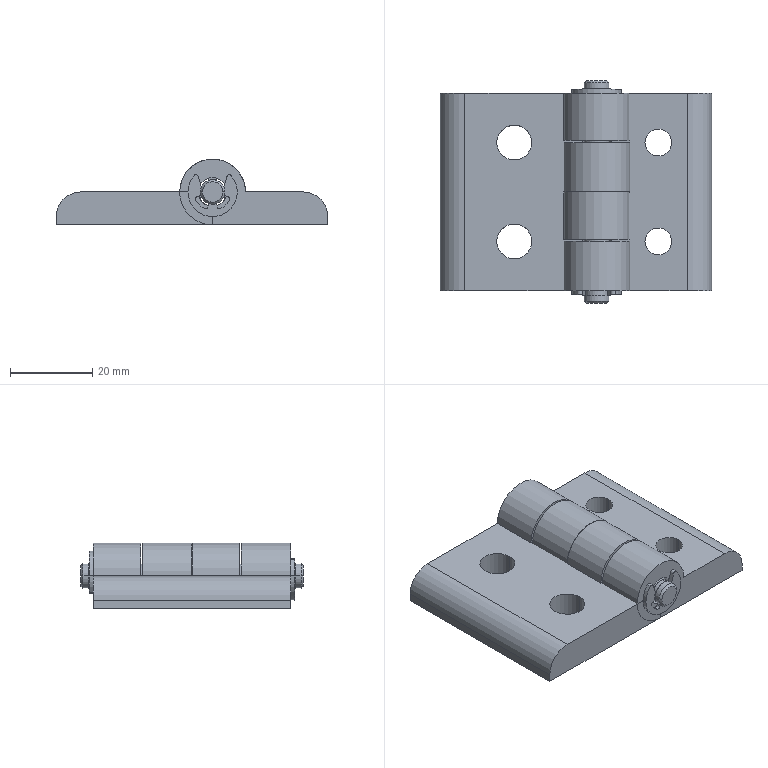Part | STEP file | aluminium hinge 30_40 (incl. half-round hex socket bolt) | 5 solids | 108 faces | box 66 x 54 x 16 mm | volume 29588 mm3 | cylinder 62 | plane 42 | cone 4 | commonest cylinder face diameters 1.2 x14 6 x14 12 x8 7 x6 5.6 x4 6.5 x4